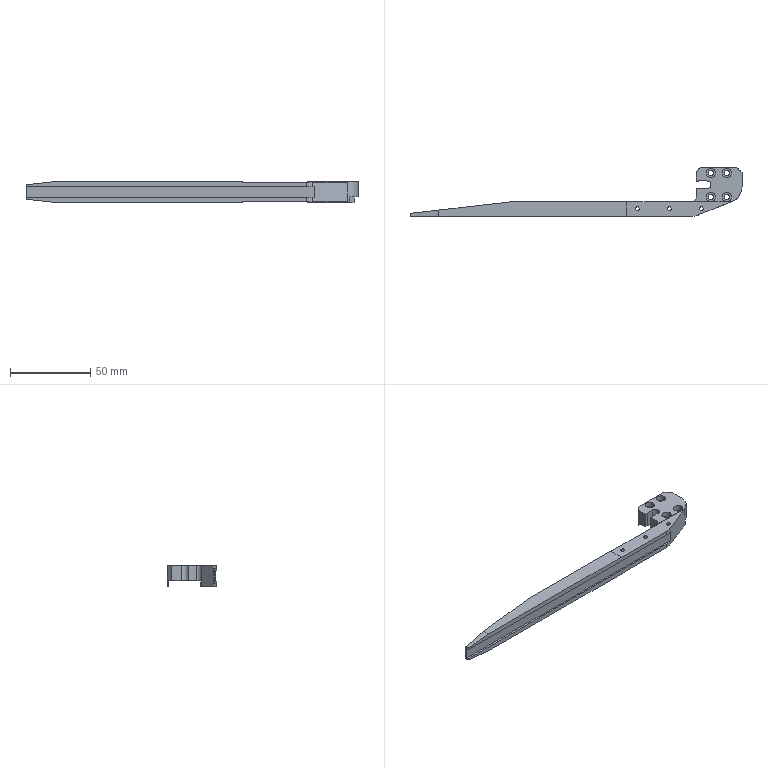NC program | NX | posted by the shop | part box 207.5 x 30.8 x 13 mm
Whole program:
%
O0001
(Machine time: 1.65 MIN)
(===Total Tool:3===)
(T6=D6      D=6.   R=0.   D-  H06 Z=-0.9  )
(T2=D6 chamfer cutter   D=6.   R=0.   D-  H02 Z=-0.5  )
(T7=D6-J    D=6.   R=0.   D7  H07 Z=-1.   )
G80 G90 G17 G49 G40
G91 G28 Z0
M01
N1 T06 M06
(D6  D=6. R=0. H=06 ce=0.10 di=0.10)
G00 G90 G54 X109.75 Y0.0 M03 S8000
G43 H06 Z10.1
M08
Z1.05
G01 Z-.45 F2000.
X106.69
Y-.39
X-79.19
Y.39
X-79.1
X106.69
Y0.0
Y-.39
X106.58
X109.75 Y-.386
Z1.05
G00 X109.845 Y0.0
Z.6
G01 Z-.9
X106.69
Y-.39
X-79.19
Y.39
X-79.1
X106.69
Y0.0
Y-.39
X106.58
X109.845
Z.6
G00 Z10.1
G91 G28 Z0.0
M05
M09
G91 G28 Z0.0
M01
N2 T02 M06
(D6 chamfer cutter  D=6. R=0. H=02 ce=0.00 di=0.00)
G00 G90 G54 X-72.21 Y-2.813 M03 S6500
G43 H02 Z50.
M08
Z.708
G01 Z-.5 F1500.
G03 X-71.924 Y-3.013 I1.286 J1.532
G01 X-71.879 Y-3.043
X-71.824 Y-3.04
X102.75
X102.804 Y-3.043
X102.85 Y-3.013
G03 X103.136 Y-2.813 I-1. J1.732
G01 Z.676
G00 Z3.25
Y2.813
Z.676
G01 Z-.5
G03 X102.85 Y3.013 I-1.286 J-1.532
G01 X102.804 Y3.043
X102.75 Y3.04
X-71.824
X-71.879 Y3.043
X-71.924 Y3.013
G03 X-72.21 Y2.813 I1. J-1.732
G01 Z.708
G00 Z50.
G91 G28 Z0.0
M05
M09
G91 G28 Z0.0
M01
N3 T07 M06
(D6-J  D=6. R=0. H=07 ce=0.00 di=0.00)
G00 G90 G54 X107.95 Y-.909 M03 S8000
G43 H07 Z10.015
M08
Z0.0
G01 Z-1. F1000.
G41 D07
Y-.709
G03 X106.75 Y.49 I-1.2 J-.001
G01 X-79.25
G03 X-80.45 Y-.709 I0.0 J-1.2
G01 G40 Y-.909
Y.909
G41 D07
Y.709
G03 X-79.25 Y-.49 I1.2 J.001
G01 X106.75
G03 X107.95 Y.709 I0.0 J1.2
G01 G40 Y.909
Z0.0
G00 Z10.015
M05
M09
G91 G28 Z0.0
G91 G28 Y0.0
M30
%